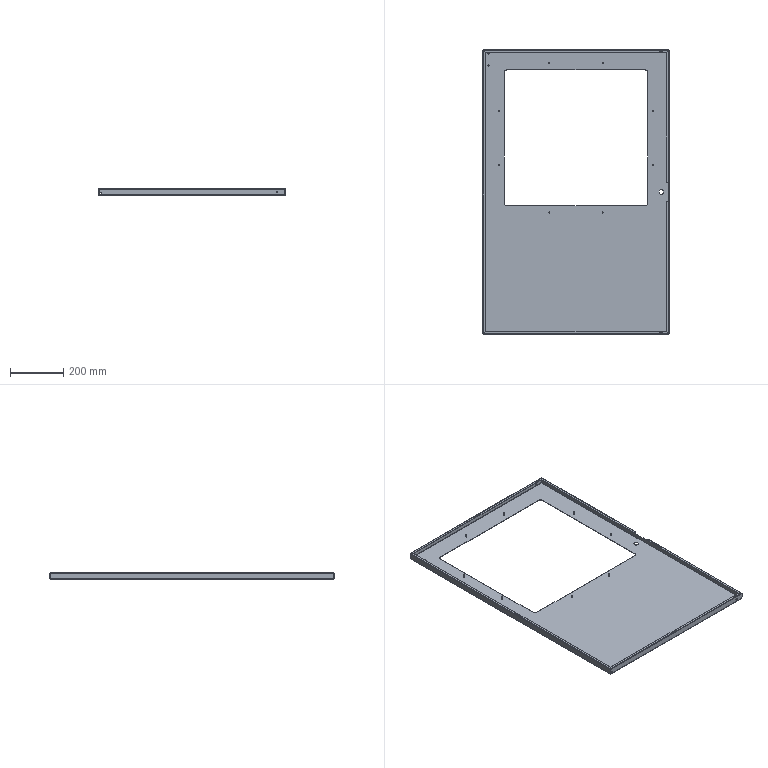Part | SolidWorks | features ICE 8, Fillet 3, EdgeFlange 2, Cut 1, FlatPattern 1, LPattern 1, MirrorPattern 1, SMBaseFlange 1, SheetMetal 1 | 1 solid | 142 faces | box 700 x 1066 x 25 mm | volume 867025 mm3 | plane 64 | cylinder 62 | spline 16 | commonest cylinder face diameters 4 x16 1.473 x9 4.473 x9 2.5 x8 5 x4 5.2 x4